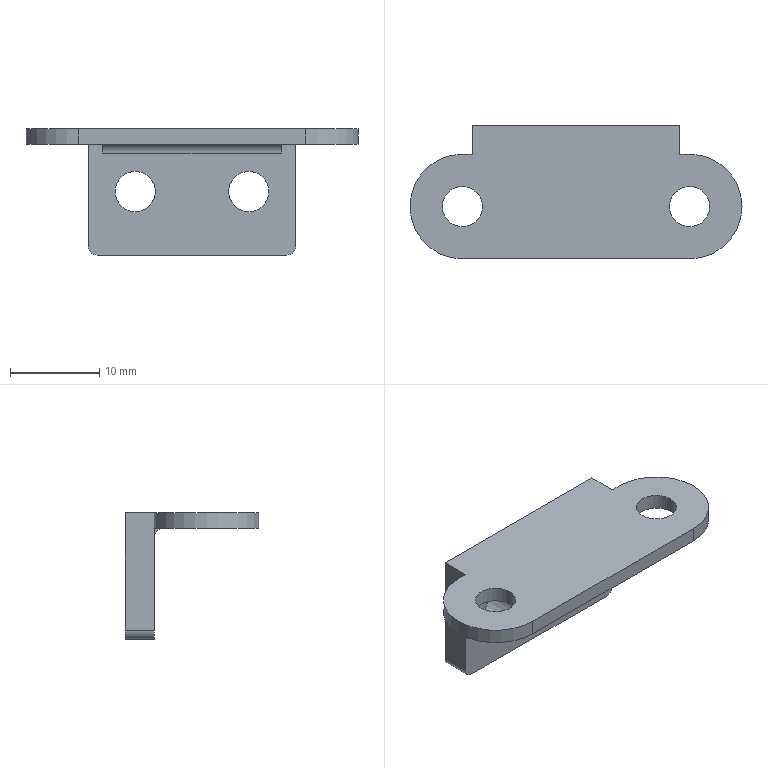Part | STEP file | CHAIN-04_1_02LT_1-2 | 1 solid | 26 faces | box 37.1 x 14.95 x 14.1 mm | volume 1597 mm3 | cylinder 14 | plane 12 | commonest cylinder face diameters 4.5 x8 2 x3 11.7 x3
STEP:
#1=CARTESIAN_POINT('',(-14.95,0.,0.));
#2=VERTEX_POINT('',#1);
#3=CARTESIAN_POINT('',(-10.45,0.,0.));
#4=VERTEX_POINT('',#3);
#5=CARTESIAN_POINT('',(-12.7,0.,0.));
#6=DIRECTION('',(0.,0.,1.));
#7=DIRECTION('',(1.,0.,0.));
#8=AXIS2_PLACEMENT_3D('',#5,#6,#7);
#9=CIRCLE('',#8,2.25);
#10=EDGE_CURVE('',#2,#4,#9,.T.);
#11=ORIENTED_EDGE('',*,*,#10,.F.);
#12=CARTESIAN_POINT('',(-14.95,0.,1.7));
#13=VERTEX_POINT('',#12);
#14=CARTESIAN_POINT('',(-14.95,0.,0.));
#15=DIRECTION('',(0.,0.,1.));
#16=VECTOR('',#15,1000.);
#17=LINE('',#14,#16);
#18=EDGE_CURVE('',#2,#13,#17,.T.);
#19=ORIENTED_EDGE('',*,*,#18,.T.);
#20=CARTESIAN_POINT('',(-10.45,0.,1.7));
#21=VERTEX_POINT('',#20);
#22=CARTESIAN_POINT('',(-12.7,0.,1.7));
#23=DIRECTION('',(0.,0.,-1.));
#24=DIRECTION('',(1.,0.,0.));
#25=AXIS2_PLACEMENT_3D('',#22,#23,#24);
#26=CIRCLE('',#25,2.25);
#27=EDGE_CURVE('',#21,#13,#26,.T.);
#28=ORIENTED_EDGE('',*,*,#27,.F.);
#29=CARTESIAN_POINT('',(-10.45,0.,0.));
#30=DIRECTION('',(0.,0.,1.));
#31=VECTOR('',#30,1000.);
#32=LINE('',#29,#31);
#33=EDGE_CURVE('',#4,#21,#32,.T.);
#34=ORIENTED_EDGE('',*,*,#33,.F.);
#35=EDGE_LOOP('',(#11,#19,#28,#34));
#36=FACE_OUTER_BOUND('',#35,.T.);
#37=CARTESIAN_POINT('',(-12.7,0.,0.));
#38=DIRECTION('',(0.,0.,1.));
#39=DIRECTION('',(1.,0.,0.));
#40=AXIS2_PLACEMENT_3D('',#37,#38,#39);
#41=CYLINDRICAL_SURFACE('',#40,2.25);
#42=ADVANCED_FACE('',(#36),#41,.F.);
#43=CARTESIAN_POINT('',(10.45,0.,0.));
#44=VERTEX_POINT('',#43);
#45=CARTESIAN_POINT('',(14.95,0.,0.));
#46=VERTEX_POINT('',#45);
#47=CARTESIAN_POINT('',(12.7,0.,0.));
#48=DIRECTION('',(0.,0.,1.));
#49=DIRECTION('',(1.,0.,0.));
#50=AXIS2_PLACEMENT_3D('',#47,#48,#49);
#51=CIRCLE('',#50,2.25);
#52=EDGE_CURVE('',#44,#46,#51,.T.);
#53=ORIENTED_EDGE('',*,*,#52,.F.);
#54=CARTESIAN_POINT('',(10.45,0.,1.7));
#55=VERTEX_POINT('',#54);
#56=CARTESIAN_POINT('',(10.45,0.,0.));
#57=DIRECTION('',(0.,0.,1.));
#58=VECTOR('',#57,1000.);
#59=LINE('',#56,#58);
#60=EDGE_CURVE('',#44,#55,#59,.T.);
#61=ORIENTED_EDGE('',*,*,#60,.T.);
#62=CARTESIAN_POINT('',(14.95,0.,1.7));
#63=VERTEX_POINT('',#62);
#64=CARTESIAN_POINT('',(12.7,0.,1.7));
#65=DIRECTION('',(0.,0.,-1.));
#66=DIRECTION('',(1.,0.,0.));
#67=AXIS2_PLACEMENT_3D('',#64,#65,#66);
#68=CIRCLE('',#67,2.25);
#69=EDGE_CURVE('',#63,#55,#68,.T.);
#70=ORIENTED_EDGE('',*,*,#69,.F.);
#71=CARTESIAN_POINT('',(14.95,0.,0.));
#72=DIRECTION('',(0.,0.,1.));
#73=VECTOR('',#72,1000.);
#74=LINE('',#71,#73);
#75=EDGE_CURVE('',#46,#63,#74,.T.);
#76=ORIENTED_EDGE('',*,*,#75,.F.);
#77=EDGE_LOOP('',(#53,#61,#70,#76));
#78=FACE_OUTER_BOUND('',#77,.T.);
#79=CARTESIAN_POINT('',(12.7,0.,0.));
#80=DIRECTION('',(0.,0.,1.));
#81=DIRECTION('',(1.,0.,0.));
#82=AXIS2_PLACEMENT_3D('',#79,#80,#81);
#83=CYLINDRICAL_SURFACE('',#82,2.25);
#84=ADVANCED_FACE('',(#78),#83,.F.);
#85=CARTESIAN_POINT('',(12.7,-5.85,0.));
#86=VERTEX_POINT('',#85);
#87=CARTESIAN_POINT('',(18.55,0.,0.));
#88=VERTEX_POINT('',#87);
#89=CARTESIAN_POINT('',(12.7,0.,0.));
#90=DIRECTION('',(0.,0.,1.));
#91=DIRECTION('',(1.,0.,0.));
#92=AXIS2_PLACEMENT_3D('',#89,#90,#91);
#93=CIRCLE('',#92,5.85);
#94=EDGE_CURVE('',#86,#88,#93,.T.);
#95=ORIENTED_EDGE('',*,*,#94,.T.);
#96=CARTESIAN_POINT('',(18.55,0.,1.7));
#97=VERTEX_POINT('',#96);
#98=CARTESIAN_POINT('',(18.55,0.,0.));
#99=DIRECTION('',(0.,0.,1.));
#100=VECTOR('',#99,1000.);
#101=LINE('',#98,#100);
#102=EDGE_CURVE('',#88,#97,#101,.T.);
#103=ORIENTED_EDGE('',*,*,#102,.T.);
#104=CARTESIAN_POINT('',(12.7,-5.85,1.7));
#105=VERTEX_POINT('',#104);
#106=CARTESIAN_POINT('',(12.7,0.,1.7));
#107=DIRECTION('',(0.,0.,1.));
#108=DIRECTION('',(1.,0.,0.));
#109=AXIS2_PLACEMENT_3D('',#106,#107,#108);
#110=CIRCLE('',#109,5.85);
#111=EDGE_CURVE('',#105,#97,#110,.T.);
#112=ORIENTED_EDGE('',*,*,#111,.F.);
#113=CARTESIAN_POINT('',(12.7,-5.85,0.));
#114=DIRECTION('',(0.,0.,-1.));
#115=VECTOR('',#114,1000.);
#116=LINE('',#113,#115);
#117=EDGE_CURVE('',#105,#86,#116,.T.);
#118=ORIENTED_EDGE('',*,*,#117,.T.);
#119=EDGE_LOOP('',(#95,#103,#112,#118));
#120=FACE_OUTER_BOUND('',#119,.T.);
#121=CARTESIAN_POINT('',(12.7,0.,0.));
#122=DIRECTION('',(0.,0.,1.));
#123=DIRECTION('',(1.,0.,0.));
#124=AXIS2_PLACEMENT_3D('',#121,#122,#123);
#125=CYLINDRICAL_SURFACE('',#124,5.85);
#126=ADVANCED_FACE('',(#120),#125,.T.);
#127=CARTESIAN_POINT('',(6.35,5.85,-3.05));
#128=VERTEX_POINT('',#127);
#129=CARTESIAN_POINT('',(6.35,5.85,-7.55));
#130=VERTEX_POINT('',#129);
#131=CARTESIAN_POINT('',(6.35,5.85,-5.3));
#132=DIRECTION('',(0.,-1.,0.));
#133=DIRECTION('',(0.,0.,1.));
#134=AXIS2_PLACEMENT_3D('',#131,#132,#133);
#135=CIRCLE('',#134,2.25);
#136=EDGE_CURVE('',#128,#130,#135,.T.);
#137=ORIENTED_EDGE('',*,*,#136,.T.);
#138=CARTESIAN_POINT('',(6.35,9.1,-7.55));
#139=VERTEX_POINT('',#138);
#140=CARTESIAN_POINT('',(6.35,9.1,-7.55));
#141=DIRECTION('',(0.,1.,0.));
#142=VECTOR('',#141,1000.);
#143=LINE('',#140,#142);
#144=EDGE_CURVE('',#130,#139,#143,.T.);
#145=ORIENTED_EDGE('',*,*,#144,.T.);
#146=CARTESIAN_POINT('',(6.35,9.1,-3.05));
#147=VERTEX_POINT('',#146);
#148=CARTESIAN_POINT('',(6.35,9.1,-5.3));
#149=DIRECTION('',(0.,1.,0.));
#150=DIRECTION('',(0.,0.,1.));
#151=AXIS2_PLACEMENT_3D('',#148,#149,#150);
#152=CIRCLE('',#151,2.25);
#153=EDGE_CURVE('',#139,#147,#152,.T.);
#154=ORIENTED_EDGE('',*,*,#153,.T.);
#155=CARTESIAN_POINT('',(6.35,9.1,-3.05));
#156=DIRECTION('',(0.,1.,0.));
#157=VECTOR('',#156,1000.);
#158=LINE('',#155,#157);
#159=EDGE_CURVE('',#128,#147,#158,.T.);
#160=ORIENTED_EDGE('',*,*,#159,.F.);
#161=EDGE_LOOP('',(#137,#145,#154,#160));
#162=FACE_OUTER_BOUND('',#161,.T.);
#163=CARTESIAN_POINT('',(6.35,9.1,-5.3));
#164=DIRECTION('',(0.,1.,0.));
#165=DIRECTION('',(0.,0.,1.));
#166=AXIS2_PLACEMENT_3D('',#163,#164,#165);
#167=CYLINDRICAL_SURFACE('',#166,2.25);
#168=ADVANCED_FACE('',(#162),#167,.F.);
#169=CARTESIAN_POINT('',(-6.35,5.85,-3.05));
#170=VERTEX_POINT('',#169);
#171=CARTESIAN_POINT('',(-6.35,5.85,-7.55));
#172=VERTEX_POINT('',#171);
#173=CARTESIAN_POINT('',(-6.35,5.85,-5.3));
#174=DIRECTION('',(0.,-1.,0.));
#175=DIRECTION('',(0.,0.,1.));
#176=AXIS2_PLACEMENT_3D('',#173,#174,#175);
#177=CIRCLE('',#176,2.25);
#178=EDGE_CURVE('',#170,#172,#177,.T.);
#179=ORIENTED_EDGE('',*,*,#178,.T.);
#180=CARTESIAN_POINT('',(-6.35,9.1,-7.55));
#181=VERTEX_POINT('',#180);
#182=CARTESIAN_POINT('',(-6.35,9.1,-7.55));
#183=DIRECTION('',(0.,1.,0.));
#184=VECTOR('',#183,1000.);
#185=LINE('',#182,#184);
#186=EDGE_CURVE('',#172,#181,#185,.T.);
#187=ORIENTED_EDGE('',*,*,#186,.T.);
#188=CARTESIAN_POINT('',(-6.35,9.1,-3.05));
#189=VERTEX_POINT('',#188);
#190=CARTESIAN_POINT('',(-6.35,9.1,-5.3));
#191=DIRECTION('',(0.,1.,0.));
#192=DIRECTION('',(0.,0.,1.));
#193=AXIS2_PLACEMENT_3D('',#190,#191,#192);
#194=CIRCLE('',#193,2.25);
#195=EDGE_CURVE('',#181,#189,#194,.T.);
#196=ORIENTED_EDGE('',*,*,#195,.T.);
#197=CARTESIAN_POINT('',(-6.35,9.1,-3.05));
#198=DIRECTION('',(0.,1.,0.));
#199=VECTOR('',#198,1000.);
#200=LINE('',#197,#199);
#201=EDGE_CURVE('',#170,#189,#200,.T.);
#202=ORIENTED_EDGE('',*,*,#201,.F.);
#203=EDGE_LOOP('',(#179,#187,#196,#202));
#204=FACE_OUTER_BOUND('',#203,.T.);
#205=CARTESIAN_POINT('',(-6.35,9.1,-5.3));
#206=DIRECTION('',(0.,1.,0.));
#207=DIRECTION('',(0.,0.,1.));
#208=AXIS2_PLACEMENT_3D('',#205,#206,#207);
#209=CYLINDRICAL_SURFACE('',#208,2.25);
#210=ADVANCED_FACE('',(#204),#209,.F.);
#211=ORIENTED_EDGE('',*,*,#27,.T.);
#212=CARTESIAN_POINT('',(-12.7,0.,1.7));
#213=DIRECTION('',(0.,0.,-1.));
#214=DIRECTION('',(1.,0.,0.));
#215=AXIS2_PLACEMENT_3D('',#212,#213,#214);
#216=CIRCLE('',#215,2.25);
#217=EDGE_CURVE('',#13,#21,#216,.T.);
#218=ORIENTED_EDGE('',*,*,#217,.T.);
#219=EDGE_LOOP('',(#211,#218));
#220=FACE_BOUND('',#219,.T.);
#221=ORIENTED_EDGE('',*,*,#69,.T.);
#222=CARTESIAN_POINT('',(12.7,0.,1.7));
#223=DIRECTION('',(0.,0.,-1.));
#224=DIRECTION('',(1.,0.,0.));
#225=AXIS2_PLACEMENT_3D('',#222,#223,#224);
#226=CIRCLE('',#225,2.25);
#227=EDGE_CURVE('',#55,#63,#226,.T.);
#228=ORIENTED_EDGE('',*,*,#227,.T.);
#229=EDGE_LOOP('',(#221,#228));
#230=FACE_BOUND('',#229,.T.);
#231=CARTESIAN_POINT('',(11.6,9.1,1.7));
#232=VERTEX_POINT('',#231);
#233=CARTESIAN_POINT('',(-11.6,9.1,1.7));
#234=VERTEX_POINT('',#233);
#235=CARTESIAN_POINT('',(0.,9.1,1.7));
#236=DIRECTION('',(-1.,0.,0.));
#237=VECTOR('',#236,1000.);
#238=LINE('',#235,#237);
#239=EDGE_CURVE('',#232,#234,#238,.T.);
#240=ORIENTED_EDGE('',*,*,#239,.T.);
#241=CARTESIAN_POINT('',(-11.6,5.85,1.7));
#242=VERTEX_POINT('',#241);
#243=CARTESIAN_POINT('',(-11.6,0.,1.7));
#244=DIRECTION('',(0.,-1.,0.));
#245=VECTOR('',#244,1000.);
#246=LINE('',#243,#245);
#247=EDGE_CURVE('',#234,#242,#246,.T.);
#248=ORIENTED_EDGE('',*,*,#247,.T.);
#249=CARTESIAN_POINT('',(-12.7,5.85,1.7));
#250=VERTEX_POINT('',#249);
#251=CARTESIAN_POINT('',(0.,5.85,1.7));
#252=DIRECTION('',(-1.,0.,0.));
#253=VECTOR('',#252,1000.);
#254=LINE('',#251,#253);
#255=EDGE_CURVE('',#242,#250,#254,.T.);
#256=ORIENTED_EDGE('',*,*,#255,.T.);
#257=CARTESIAN_POINT('',(-12.7,-5.85,1.7));
#258=VERTEX_POINT('',#257);
#259=CARTESIAN_POINT('',(-12.7,0.,1.7));
#260=DIRECTION('',(0.,0.,1.));
#261=DIRECTION('',(1.,0.,0.));
#262=AXIS2_PLACEMENT_3D('',#259,#260,#261);
#263=CIRCLE('',#262,5.85);
#264=EDGE_CURVE('',#250,#258,#263,.T.);
#265=ORIENTED_EDGE('',*,*,#264,.T.);
#266=CARTESIAN_POINT('',(0.,-5.85,1.7));
#267=DIRECTION('',(1.,0.,0.));
#268=VECTOR('',#267,1000.);
#269=LINE('',#266,#268);
#270=EDGE_CURVE('',#258,#105,#269,.T.);
#271=ORIENTED_EDGE('',*,*,#270,.T.);
#272=ORIENTED_EDGE('',*,*,#111,.T.);
#273=CARTESIAN_POINT('',(12.7,5.85,1.7));
#274=VERTEX_POINT('',#273);
#275=CARTESIAN_POINT('',(12.7,0.,1.7));
#276=DIRECTION('',(0.,0.,1.));
#277=DIRECTION('',(1.,0.,0.));
#278=AXIS2_PLACEMENT_3D('',#275,#276,#277);
#279=CIRCLE('',#278,5.85);
#280=EDGE_CURVE('',#97,#274,#279,.T.);
#281=ORIENTED_EDGE('',*,*,#280,.T.);
#282=CARTESIAN_POINT('',(11.6,5.85,1.7));
#283=VERTEX_POINT('',#282);
#284=CARTESIAN_POINT('',(0.,5.85,1.7));
#285=DIRECTION('',(-1.,0.,0.));
#286=VECTOR('',#285,1000.);
#287=LINE('',#284,#286);
#288=EDGE_CURVE('',#274,#283,#287,.T.);
#289=ORIENTED_EDGE('',*,*,#288,.T.);
#290=CARTESIAN_POINT('',(11.6,0.,1.7));
#291=DIRECTION('',(0.,1.,0.));
#292=VECTOR('',#291,1000.);
#293=LINE('',#290,#292);
#294=EDGE_CURVE('',#283,#232,#293,.T.);
#295=ORIENTED_EDGE('',*,*,#294,.T.);
#296=EDGE_LOOP('',(#240,#248,#256,#265,#271,#272,#281,#289,#295));
#297=FACE_OUTER_BOUND('',#296,.T.);
#298=CARTESIAN_POINT('',(0.,0.,1.7));
#299=DIRECTION('',(0.,0.,1.));
#300=DIRECTION('',(1.,0.,0.));
#301=AXIS2_PLACEMENT_3D('',#298,#299,#300);
#302=PLANE('',#301);
#303=ADVANCED_FACE('',(#220,#230,#297),#302,.T.);
#304=ORIENTED_EDGE('',*,*,#18,.F.);
#305=CARTESIAN_POINT('',(-12.7,0.,0.));
#306=DIRECTION('',(0.,0.,1.));
#307=DIRECTION('',(1.,0.,0.));
#308=AXIS2_PLACEMENT_3D('',#305,#306,#307);
#309=CIRCLE('',#308,2.25);
#310=EDGE_CURVE('',#4,#2,#309,.T.);
#311=ORIENTED_EDGE('',*,*,#310,.F.);
#312=ORIENTED_EDGE('',*,*,#33,.T.);
#313=ORIENTED_EDGE('',*,*,#217,.F.);
#314=EDGE_LOOP('',(#304,#311,#312,#313));
#315=FACE_OUTER_BOUND('',#314,.T.);
#316=CARTESIAN_POINT('',(-12.7,0.,0.));
#317=DIRECTION('',(0.,0.,1.));
#318=DIRECTION('',(1.,0.,0.));
#319=AXIS2_PLACEMENT_3D('',#316,#317,#318);
#320=CYLINDRICAL_SURFACE('',#319,2.25);
#321=ADVANCED_FACE('',(#315),#320,.F.);
#322=ORIENTED_EDGE('',*,*,#60,.F.);
#323=CARTESIAN_POINT('',(12.7,0.,0.));
#324=DIRECTION('',(0.,0.,1.));
#325=DIRECTION('',(1.,0.,0.));
#326=AXIS2_PLACEMENT_3D('',#323,#324,#325);
#327=CIRCLE('',#326,2.25);
#328=EDGE_CURVE('',#46,#44,#327,.T.);
#329=ORIENTED_EDGE('',*,*,#328,.F.);
#330=ORIENTED_EDGE('',*,*,#75,.T.);
#331=ORIENTED_EDGE('',*,*,#227,.F.);
#332=EDGE_LOOP('',(#322,#329,#330,#331));
#333=FACE_OUTER_BOUND('',#332,.T.);
#334=CARTESIAN_POINT('',(12.7,0.,0.));
#335=DIRECTION('',(0.,0.,1.));
#336=DIRECTION('',(1.,0.,0.));
#337=AXIS2_PLACEMENT_3D('',#334,#335,#336);
#338=CYLINDRICAL_SURFACE('',#337,2.25);
#339=ADVANCED_FACE('',(#333),#338,.F.);
#340=CARTESIAN_POINT('',(-11.6,5.85,0.));
#341=VERTEX_POINT('',#340);
#342=CARTESIAN_POINT('',(-11.6,5.85,-11.4));
#343=VERTEX_POINT('',#342);
#344=CARTESIAN_POINT('',(-11.6,5.85,1.7));
#345=DIRECTION('',(0.,0.,-1.));
#346=VECTOR('',#345,1000.);
#347=LINE('',#344,#346);
#348=EDGE_CURVE('',#341,#343,#347,.T.);
#349=ORIENTED_EDGE('',*,*,#348,.F.);
#350=CARTESIAN_POINT('',(-11.6,5.85,1.7));
#351=DIRECTION('',(0.,0.,-1.));
#352=VECTOR('',#351,1000.);
#353=LINE('',#350,#352);
#354=EDGE_CURVE('',#242,#341,#353,.T.);
#355=ORIENTED_EDGE('',*,*,#354,.F.);
#356=ORIENTED_EDGE('',*,*,#247,.F.);
#357=CARTESIAN_POINT('',(-11.6,9.1,-11.4));
#358=VERTEX_POINT('',#357);
#359=CARTESIAN_POINT('',(-11.6,9.1,1.7));
#360=DIRECTION('',(0.,0.,1.));
#361=VECTOR('',#360,1000.);
#362=LINE('',#359,#361);
#363=EDGE_CURVE('',#358,#234,#362,.T.);
#364=ORIENTED_EDGE('',*,*,#363,.F.);
#365=CARTESIAN_POINT('',(-11.6,9.1,-11.4));
#366=DIRECTION('',(0.,1.,0.));
#367=VECTOR('',#366,1000.);
#368=LINE('',#365,#367);
#369=EDGE_CURVE('',#343,#358,#368,.T.);
#370=ORIENTED_EDGE('',*,*,#369,.F.);
#371=EDGE_LOOP('',(#349,#355,#356,#364,#370));
#372=FACE_OUTER_BOUND('',#371,.T.);
#373=CARTESIAN_POINT('',(-11.6,9.1,1.7));
#374=DIRECTION('',(1.,0.,0.));
#375=DIRECTION('',(0.,0.,-1.));
#376=AXIS2_PLACEMENT_3D('',#373,#374,#375);
#377=PLANE('',#376);
#378=ADVANCED_FACE('',(#372),#377,.F.);
#379=CARTESIAN_POINT('',(6.35,9.1,-5.3));
#380=DIRECTION('',(0.,1.,0.));
#381=DIRECTION('',(0.,0.,1.));
#382=AXIS2_PLACEMENT_3D('',#379,#380,#381);
#383=CIRCLE('',#382,2.25);
#384=EDGE_CURVE('',#147,#139,#383,.T.);
#385=ORIENTED_EDGE('',*,*,#384,.F.);
#386=ORIENTED_EDGE('',*,*,#153,.F.);
#387=EDGE_LOOP('',(#385,#386));
#388=FACE_BOUND('',#387,.T.);
#389=CARTESIAN_POINT('',(-6.35,9.1,-5.3));
#390=DIRECTION('',(0.,1.,0.));
#391=DIRECTION('',(0.,0.,1.));
#392=AXIS2_PLACEMENT_3D('',#389,#390,#391);
#393=CIRCLE('',#392,2.25);
#394=EDGE_CURVE('',#189,#181,#393,.T.);
#395=ORIENTED_EDGE('',*,*,#394,.F.);
#396=ORIENTED_EDGE('',*,*,#195,.F.);
#397=EDGE_LOOP('',(#395,#396));
#398=FACE_BOUND('',#397,.T.);
#399=CARTESIAN_POINT('',(-10.6,9.1,-12.4));
#400=VERTEX_POINT('',#399);
#401=CARTESIAN_POINT('',(10.6,9.1,-12.4));
#402=VERTEX_POINT('',#401);
#403=CARTESIAN_POINT('',(-11.6,9.1,-12.4));
#404=DIRECTION('',(1.,0.,0.));
#405=VECTOR('',#404,1000.);
#406=LINE('',#403,#405);
#407=EDGE_CURVE('',#400,#402,#406,.T.);
#408=ORIENTED_EDGE('',*,*,#407,.F.);
#409=CARTESIAN_POINT('',(-10.6,9.1,-11.4));
#410=DIRECTION('',(0.,-1.,0.));
#411=DIRECTION('',(0.,0.,-1.));
#412=AXIS2_PLACEMENT_3D('',#409,#410,#411);
#413=CIRCLE('',#412,1.);
#414=EDGE_CURVE('',#358,#400,#413,.T.);
#415=ORIENTED_EDGE('',*,*,#414,.F.);
#416=ORIENTED_EDGE('',*,*,#363,.T.);
#417=ORIENTED_EDGE('',*,*,#239,.F.);
#418=CARTESIAN_POINT('',(11.6,9.1,-11.4));
#419=VERTEX_POINT('',#418);
#420=CARTESIAN_POINT('',(11.6,9.1,-12.4));
#421=DIRECTION('',(0.,0.,1.));
#422=VECTOR('',#421,1000.);
#423=LINE('',#420,#422);
#424=EDGE_CURVE('',#419,#232,#423,.T.);
#425=ORIENTED_EDGE('',*,*,#424,.F.);
#426=CARTESIAN_POINT('',(10.6,9.1,-11.4));
#427=DIRECTION('',(0.,-1.,0.));
#428=DIRECTION('',(0.,0.,-1.));
#429=AXIS2_PLACEMENT_3D('',#426,#427,#428);
#430=CIRCLE('',#429,1.);
#431=EDGE_CURVE('',#402,#419,#430,.T.);
#432=ORIENTED_EDGE('',*,*,#431,.F.);
#433=EDGE_LOOP('',(#408,#415,#416,#417,#425,#432));
#434=FACE_OUTER_BOUND('',#433,.T.);
#435=CARTESIAN_POINT('',(-11.6,9.1,-12.4));
#436=DIRECTION('',(0.,-1.,0.));
#437=DIRECTION('',(0.,0.,-1.));
#438=AXIS2_PLACEMENT_3D('',#435,#436,#437);
#439=PLANE('',#438);
#440=ADVANCED_FACE('',(#388,#398,#434),#439,.F.);
#441=ORIENTED_EDGE('',*,*,#424,.T.);
#442=ORIENTED_EDGE('',*,*,#294,.F.);
#443=CARTESIAN_POINT('',(11.6,5.85,0.));
#444=VERTEX_POINT('',#443);
#445=CARTESIAN_POINT('',(11.6,5.85,1.7));
#446=DIRECTION('',(0.,0.,1.));
#447=VECTOR('',#446,1000.);
#448=LINE('',#445,#447);
#449=EDGE_CURVE('',#444,#283,#448,.T.);
#450=ORIENTED_EDGE('',*,*,#449,.F.);
#451=CARTESIAN_POINT('',(11.6,5.85,-11.4));
#452=VERTEX_POINT('',#451);
#453=CARTESIAN_POINT('',(11.6,5.85,1.7));
#454=DIRECTION('',(0.,0.,1.));
#455=VECTOR('',#454,1000.);
#456=LINE('',#453,#455);
#457=EDGE_CURVE('',#452,#444,#456,.T.);
#458=ORIENTED_EDGE('',*,*,#457,.F.);
#459=CARTESIAN_POINT('',(11.6,9.1,-11.4));
#460=DIRECTION('',(0.,-1.,0.));
#461=VECTOR('',#460,1000.);
#462=LINE('',#459,#461);
#463=EDGE_CURVE('',#419,#452,#462,.T.);
#464=ORIENTED_EDGE('',*,*,#463,.F.);
#465=EDGE_LOOP('',(#441,#442,#450,#458,#464));
#466=FACE_OUTER_BOUND('',#465,.T.);
#467=CARTESIAN_POINT('',(11.6,9.1,1.7));
#468=DIRECTION('',(-1.,0.,0.));
#469=DIRECTION('',(0.,0.,1.));
#470=AXIS2_PLACEMENT_3D('',#467,#468,#469);
#471=PLANE('',#470);
#472=ADVANCED_FACE('',(#466),#471,.F.);
#473=CARTESIAN_POINT('',(12.7,5.85,0.));
#474=VERTEX_POINT('',#473);
#475=CARTESIAN_POINT('',(12.7,5.85,0.));
#476=DIRECTION('',(0.,0.,-1.));
#477=VECTOR('',#476,1000.);
#478=LINE('',#475,#477);
#479=EDGE_CURVE('',#274,#474,#478,.T.);
#480=ORIENTED_EDGE('',*,*,#479,.T.);
#481=CARTESIAN_POINT('',(12.7,5.85,0.));
#482=DIRECTION('',(-1.,0.,0.));
#483=VECTOR('',#482,1000.);
#484=LINE('',#481,#483);
#485=EDGE_CURVE('',#474,#444,#484,.T.);
#486=ORIENTED_EDGE('',*,*,#485,.T.);
#487=ORIENTED_EDGE('',*,*,#449,.T.);
#488=ORIENTED_EDGE('',*,*,#288,.F.);
#489=EDGE_LOOP('',(#480,#486,#487,#488));
#490=FACE_OUTER_BOUND('',#489,.T.);
#491=CARTESIAN_POINT('',(12.7,5.85,0.));
#492=DIRECTION('',(0.,1.,0.));
#493=DIRECTION('',(0.,0.,1.));
#494=AXIS2_PLACEMENT_3D('',#491,#492,#493);
#495=PLANE('',#494);
#496=ADVANCED_FACE('',(#490),#495,.T.);
#497=ORIENTED_EDGE('',*,*,#102,.F.);
#498=CARTESIAN_POINT('',(12.7,0.,0.));
#499=DIRECTION('',(0.,0.,1.));
#500=DIRECTION('',(1.,0.,0.));
#501=AXIS2_PLACEMENT_3D('',#498,#499,#500);
#502=CIRCLE('',#501,5.85);
#503=EDGE_CURVE('',#88,#474,#502,.T.);
#504=ORIENTED_EDGE('',*,*,#503,.T.);
#505=ORIENTED_EDGE('',*,*,#479,.F.);
#506=ORIENTED_EDGE('',*,*,#280,.F.);
#507=EDGE_LOOP('',(#497,#504,#505,#506));
#508=FACE_OUTER_BOUND('',#507,.T.);
#509=CARTESIAN_POINT('',(12.7,0.,0.));
#510=DIRECTION('',(0.,0.,1.));
#511=DIRECTION('',(1.,0.,0.));
#512=AXIS2_PLACEMENT_3D('',#509,#510,#511);
#513=CYLINDRICAL_SURFACE('',#512,5.85);
#514=ADVANCED_FACE('',(#508),#513,.T.);
#515=ORIENTED_EDGE('',*,*,#117,.F.);
#516=ORIENTED_EDGE('',*,*,#270,.F.);
#517=CARTESIAN_POINT('',(-12.7,-5.85,0.));
#518=VERTEX_POINT('',#517);
#519=CARTESIAN_POINT('',(-12.7,-5.85,0.));
#520=DIRECTION('',(0.,0.,-1.));
#521=VECTOR('',#520,1000.);
#522=LINE('',#519,#521);
#523=EDGE_CURVE('',#258,#518,#522,.T.);
#524=ORIENTED_EDGE('',*,*,#523,.T.);
#525=CARTESIAN_POINT('',(-12.7,-5.85,0.));
#526=DIRECTION('',(1.,0.,0.));
#527=VECTOR('',#526,1000.);
#528=LINE('',#525,#527);
#529=EDGE_CURVE('',#518,#86,#528,.T.);
#530=ORIENTED_EDGE('',*,*,#529,.T.);
#531=EDGE_LOOP('',(#515,#516,#524,#530));
#532=FACE_OUTER_BOUND('',#531,.T.);
#533=CARTESIAN_POINT('',(-12.7,-5.85,0.));
#534=DIRECTION('',(0.,-1.,0.));
#535=DIRECTION('',(0.,0.,-1.));
#536=AXIS2_PLACEMENT_3D('',#533,#534,#535);
#537=PLANE('',#536);
#538=ADVANCED_FACE('',(#532),#537,.T.);
#539=ORIENTED_EDGE('',*,*,#523,.F.);
#540=ORIENTED_EDGE('',*,*,#264,.F.);
#541=CARTESIAN_POINT('',(-12.7,5.85,0.));
#542=VERTEX_POINT('',#541);
#543=CARTESIAN_POINT('',(-12.7,5.85,0.));
#544=DIRECTION('',(0.,0.,-1.));
#545=VECTOR('',#544,1000.);
#546=LINE('',#543,#545);
#547=EDGE_CURVE('',#250,#542,#546,.T.);
#548=ORIENTED_EDGE('',*,*,#547,.T.);
#549=CARTESIAN_POINT('',(-12.7,0.,0.));
#550=DIRECTION('',(0.,0.,1.));
#551=DIRECTION('',(1.,0.,0.));
#552=AXIS2_PLACEMENT_3D('',#549,#550,#551);
#553=CIRCLE('',#552,5.85);
#554=EDGE_CURVE('',#542,#518,#553,.T.);
#555=ORIENTED_EDGE('',*,*,#554,.T.);
#556=EDGE_LOOP('',(#539,#540,#548,#555));
#557=FACE_OUTER_BOUND('',#556,.T.);
#558=CARTESIAN_POINT('',(-12.7,0.,0.));
#559=DIRECTION('',(0.,0.,1.));
#560=DIRECTION('',(1.,0.,0.));
#561=AXIS2_PLACEMENT_3D('',#558,#559,#560);
#562=CYLINDRICAL_SURFACE('',#561,5.85);
#563=ADVANCED_FACE('',(#557),#562,.T.);
#564=ORIENTED_EDGE('',*,*,#547,.F.);
#565=ORIENTED_EDGE('',*,*,#255,.F.);
#566=ORIENTED_EDGE('',*,*,#354,.T.);
#567=CARTESIAN_POINT('',(12.7,5.85,0.));
#568=DIRECTION('',(-1.,0.,0.));
#569=VECTOR('',#568,1000.);
#570=LINE('',#567,#569);
#571=EDGE_CURVE('',#341,#542,#570,.T.);
#572=ORIENTED_EDGE('',*,*,#571,.T.);
#573=EDGE_LOOP('',(#564,#565,#566,#572));
#574=FACE_OUTER_BOUND('',#573,.T.);
#575=CARTESIAN_POINT('',(12.7,5.85,0.));
#576=DIRECTION('',(0.,1.,0.));
#577=DIRECTION('',(0.,0.,1.));
#578=AXIS2_PLACEMENT_3D('',#575,#576,#577);
#579=PLANE('',#578);
#580=ADVANCED_FACE('',(#574),#579,.T.);
#581=ORIENTED_EDGE('',*,*,#310,.T.);
#582=ORIENTED_EDGE('',*,*,#10,.T.);
#583=EDGE_LOOP('',(#581,#582));
#584=FACE_BOUND('',#583,.T.);
#585=ORIENTED_EDGE('',*,*,#328,.T.);
#586=ORIENTED_EDGE('',*,*,#52,.T.);
#587=EDGE_LOOP('',(#585,#586));
#588=FACE_BOUND('',#587,.T.);
#589=ORIENTED_EDGE('',*,*,#554,.F.);
#590=ORIENTED_EDGE('',*,*,#571,.F.);
#591=CARTESIAN_POINT('',(-10.,5.85,0.));
#592=VERTEX_POINT('',#591);
#593=CARTESIAN_POINT('',(0.,5.85,0.));
#594=DIRECTION('',(-1.,0.,0.));
#595=VECTOR('',#594,1000.);
#596=LINE('',#593,#595);
#597=EDGE_CURVE('',#592,#341,#596,.T.);
#598=ORIENTED_EDGE('',*,*,#597,.F.);
#599=CARTESIAN_POINT('',(-10.,4.85,0.));
#600=VERTEX_POINT('',#599);
#601=CARTESIAN_POINT('',(-10.,0.,0.));
#602=DIRECTION('',(0.,1.,0.));
#603=VECTOR('',#602,1000.);
#604=LINE('',#601,#603);
#605=EDGE_CURVE('',#600,#592,#604,.T.);
#606=ORIENTED_EDGE('',*,*,#605,.F.);
#607=CARTESIAN_POINT('',(10.,4.85,0.));
#608=VERTEX_POINT('',#607);
#609=CARTESIAN_POINT('',(0.,4.85,0.));
#610=DIRECTION('',(-1.,0.,0.));
#611=VECTOR('',#610,1000.);
#612=LINE('',#609,#611);
#613=EDGE_CURVE('',#608,#600,#612,.T.);
#614=ORIENTED_EDGE('',*,*,#613,.F.);
#615=CARTESIAN_POINT('',(10.,5.85,0.));
#616=VERTEX_POINT('',#615);
#617=CARTESIAN_POINT('',(10.,0.,0.));
#618=DIRECTION('',(0.,-1.,0.));
#619=VECTOR('',#618,1000.);
#620=LINE('',#617,#619);
#621=EDGE_CURVE('',#616,#608,#620,.T.);
#622=ORIENTED_EDGE('',*,*,#621,.F.);
#623=CARTESIAN_POINT('',(0.,5.85,0.));
#624=DIRECTION('',(-1.,0.,0.));
#625=VECTOR('',#624,1000.);
#626=LINE('',#623,#625);
#627=EDGE_CURVE('',#444,#616,#626,.T.);
#628=ORIENTED_EDGE('',*,*,#627,.F.);
#629=ORIENTED_EDGE('',*,*,#485,.F.);
#630=ORIENTED_EDGE('',*,*,#503,.F.);
#631=ORIENTED_EDGE('',*,*,#94,.F.);
#632=ORIENTED_EDGE('',*,*,#529,.F.);
#633=EDGE_LOOP('',(#589,#590,#598,#606,#614,#622,#628,#629,#630,#631,#632));
#634=FACE_OUTER_BOUND('',#633,.T.);
#635=CARTESIAN_POINT('',(0.,0.,0.));
#636=DIRECTION('',(0.,0.,1.));
#637=DIRECTION('',(1.,0.,0.));
#638=AXIS2_PLACEMENT_3D('',#635,#636,#637);
#639=PLANE('',#638);
#640=ADVANCED_FACE('',(#584,#588,#634),#639,.F.);
#641=ORIENTED_EDGE('',*,*,#369,.T.);
#642=ORIENTED_EDGE('',*,*,#414,.T.);
#643=CARTESIAN_POINT('',(-10.6,5.85,-12.4));
#644=VERTEX_POINT('',#643);
#645=CARTESIAN_POINT('',(-10.6,9.1,-12.4));
#646=DIRECTION('',(0.,-1.,0.));
#647=VECTOR('',#646,1000.);
#648=LINE('',#645,#647);
#649=EDGE_CURVE('',#400,#644,#648,.T.);
#650=ORIENTED_EDGE('',*,*,#649,.T.);
#651=CARTESIAN_POINT('',(-10.6,5.85,-11.4));
#652=DIRECTION('',(0.,1.,0.));
#653=DIRECTION('',(0.,0.,-1.));
#654=AXIS2_PLACEMENT_3D('',#651,#652,#653);
#655=CIRCLE('',#654,1.);
#656=EDGE_CURVE('',#644,#343,#655,.T.);
#657=ORIENTED_EDGE('',*,*,#656,.T.);
#658=EDGE_LOOP('',(#641,#642,#650,#657));
#659=FACE_OUTER_BOUND('',#658,.T.);
#660=CARTESIAN_POINT('',(-10.6,9.1,-11.4));
#661=DIRECTION('',(0.,-1.,0.));
#662=DIRECTION('',(0.,0.,-1.));
#663=AXIS2_PLACEMENT_3D('',#660,#661,#662);
#664=CYLINDRICAL_SURFACE('',#663,1.);
#665=ADVANCED_FACE('',(#659),#664,.T.);
#666=ORIENTED_EDGE('',*,*,#136,.F.);
#667=CARTESIAN_POINT('',(6.35,5.85,-5.3));
#668=DIRECTION('',(0.,-1.,0.));
#669=DIRECTION('',(0.,0.,1.));
#670=AXIS2_PLACEMENT_3D('',#667,#668,#669);
#671=CIRCLE('',#670,2.25);
#672=EDGE_CURVE('',#130,#128,#671,.T.);
#673=ORIENTED_EDGE('',*,*,#672,.F.);
#674=EDGE_LOOP('',(#666,#673));
#675=FACE_BOUND('',#674,.T.);
#676=ORIENTED_EDGE('',*,*,#178,.F.);
#677=CARTESIAN_POINT('',(-6.35,5.85,-5.3));
#678=DIRECTION('',(0.,-1.,0.));
#679=DIRECTION('',(0.,0.,1.));
#680=AXIS2_PLACEMENT_3D('',#677,#678,#679);
#681=CIRCLE('',#680,2.25);
#682=EDGE_CURVE('',#172,#170,#681,.T.);
#683=ORIENTED_EDGE('',*,*,#682,.F.);
#684=EDGE_LOOP('',(#676,#683));
#685=FACE_BOUND('',#684,.T.);
#686=ORIENTED_EDGE('',*,*,#457,.T.);
#687=ORIENTED_EDGE('',*,*,#627,.T.);
#688=CARTESIAN_POINT('',(10.,5.85,-1.));
#689=VERTEX_POINT('',#688);
#690=CARTESIAN_POINT('',(10.,5.85,0.));
#691=DIRECTION('',(0.,0.,1.));
#692=VECTOR('',#691,1000.);
#693=LINE('',#690,#692);
#694=EDGE_CURVE('',#689,#616,#693,.T.);
#695=ORIENTED_EDGE('',*,*,#694,.F.);
#696=CARTESIAN_POINT('',(-10.,5.85,-1.));
#697=VERTEX_POINT('',#696);
#698=CARTESIAN_POINT('',(0.,5.85,-1.));
#699=DIRECTION('',(1.,0.,0.));
#700=VECTOR('',#699,1000.);
#701=LINE('',#698,#700);
#702=EDGE_CURVE('',#697,#689,#701,.T.);
#703=ORIENTED_EDGE('',*,*,#702,.F.);
#704=CARTESIAN_POINT('',(-10.,5.85,0.));
#705=DIRECTION('',(0.,0.,-1.));
#706=VECTOR('',#705,1000.);
#707=LINE('',#704,#706);
#708=EDGE_CURVE('',#592,#697,#707,.T.);
#709=ORIENTED_EDGE('',*,*,#708,.F.);
#710=ORIENTED_EDGE('',*,*,#597,.T.);
#711=ORIENTED_EDGE('',*,*,#348,.T.);
#712=ORIENTED_EDGE('',*,*,#656,.F.);
#713=CARTESIAN_POINT('',(10.6,5.85,-12.4));
#714=VERTEX_POINT('',#713);
#715=CARTESIAN_POINT('',(0.,5.85,-12.4));
#716=DIRECTION('',(-1.,0.,0.));
#717=VECTOR('',#716,1000.);
#718=LINE('',#715,#717);
#719=EDGE_CURVE('',#714,#644,#718,.T.);
#720=ORIENTED_EDGE('',*,*,#719,.F.);
#721=CARTESIAN_POINT('',(10.6,5.85,-11.4));
#722=DIRECTION('',(0.,1.,0.));
#723=DIRECTION('',(0.,0.,-1.));
#724=AXIS2_PLACEMENT_3D('',#721,#722,#723);
#725=CIRCLE('',#724,1.);
#726=EDGE_CURVE('',#452,#714,#725,.T.);
#727=ORIENTED_EDGE('',*,*,#726,.F.);
#728=EDGE_LOOP('',(#686,#687,#695,#703,#709,#710,#711,#712,#720,#727));
#729=FACE_OUTER_BOUND('',#728,.T.);
#730=CARTESIAN_POINT('',(0.,5.85,0.));
#731=DIRECTION('',(0.,1.,0.));
#732=DIRECTION('',(0.,0.,1.));
#733=AXIS2_PLACEMENT_3D('',#730,#731,#732);
#734=PLANE('',#733);
#735=ADVANCED_FACE('',(#675,#685,#729),#734,.F.);
#736=ORIENTED_EDGE('',*,*,#144,.F.);
#737=ORIENTED_EDGE('',*,*,#672,.T.);
#738=ORIENTED_EDGE('',*,*,#159,.T.);
#739=ORIENTED_EDGE('',*,*,#384,.T.);
#740=EDGE_LOOP('',(#736,#737,#738,#739));
#741=FACE_OUTER_BOUND('',#740,.T.);
#742=CARTESIAN_POINT('',(6.35,9.1,-5.3));
#743=DIRECTION('',(0.,1.,0.));
#744=DIRECTION('',(0.,0.,1.));
#745=AXIS2_PLACEMENT_3D('',#742,#743,#744);
#746=CYLINDRICAL_SURFACE('',#745,2.25);
#747=ADVANCED_FACE('',(#741),#746,.F.);
#748=ORIENTED_EDGE('',*,*,#186,.F.);
#749=ORIENTED_EDGE('',*,*,#682,.T.);
#750=ORIENTED_EDGE('',*,*,#201,.T.);
#751=ORIENTED_EDGE('',*,*,#394,.T.);
#752=EDGE_LOOP('',(#748,#749,#750,#751));
#753=FACE_OUTER_BOUND('',#752,.T.);
#754=CARTESIAN_POINT('',(-6.35,9.1,-5.3));
#755=DIRECTION('',(0.,1.,0.));
#756=DIRECTION('',(0.,0.,1.));
#757=AXIS2_PLACEMENT_3D('',#754,#755,#756);
#758=CYLINDRICAL_SURFACE('',#757,2.25);
#759=ADVANCED_FACE('',(#753),#758,.F.);
#760=ORIENTED_EDGE('',*,*,#719,.T.);
#761=ORIENTED_EDGE('',*,*,#649,.F.);
#762=ORIENTED_EDGE('',*,*,#407,.T.);
#763=CARTESIAN_POINT('',(10.6,9.1,-12.4));
#764=DIRECTION('',(0.,1.,0.));
#765=VECTOR('',#764,1000.);
#766=LINE('',#763,#765);
#767=EDGE_CURVE('',#714,#402,#766,.T.);
#768=ORIENTED_EDGE('',*,*,#767,.F.);
#769=EDGE_LOOP('',(#760,#761,#762,#768));
#770=FACE_OUTER_BOUND('',#769,.T.);
#771=CARTESIAN_POINT('',(-11.6,9.1,-12.4));
#772=DIRECTION('',(0.,0.,1.));
#773=DIRECTION('',(1.,0.,0.));
#774=AXIS2_PLACEMENT_3D('',#771,#772,#773);
#775=PLANE('',#774);
#776=ADVANCED_FACE('',(#770),#775,.F.);
#777=ORIENTED_EDGE('',*,*,#767,.T.);
#778=ORIENTED_EDGE('',*,*,#431,.T.);
#779=ORIENTED_EDGE('',*,*,#463,.T.);
#780=ORIENTED_EDGE('',*,*,#726,.T.);
#781=EDGE_LOOP('',(#777,#778,#779,#780));
#782=FACE_OUTER_BOUND('',#781,.T.);
#783=CARTESIAN_POINT('',(10.6,9.1,-11.4));
#784=DIRECTION('',(0.,-1.,0.));
#785=DIRECTION('',(0.,0.,-1.));
#786=AXIS2_PLACEMENT_3D('',#783,#784,#785);
#787=CYLINDRICAL_SURFACE('',#786,1.);
#788=ADVANCED_FACE('',(#782),#787,.T.);
#789=ORIENTED_EDGE('',*,*,#605,.T.);
#790=ORIENTED_EDGE('',*,*,#708,.T.);
#791=CARTESIAN_POINT('',(-10.,4.85,-1.));
#792=DIRECTION('',(1.,0.,0.));
#793=DIRECTION('',(0.,0.,1.));
#794=AXIS2_PLACEMENT_3D('',#791,#792,#793);
#795=CIRCLE('',#794,1.);
#796=EDGE_CURVE('',#697,#600,#795,.T.);
#797=ORIENTED_EDGE('',*,*,#796,.T.);
#798=EDGE_LOOP('',(#789,#790,#797));
#799=FACE_OUTER_BOUND('',#798,.T.);
#800=CARTESIAN_POINT('',(-10.,5.85,-11.3));
#801=DIRECTION('',(-1.,0.,0.));
#802=DIRECTION('',(0.,0.,1.));
#803=AXIS2_PLACEMENT_3D('',#800,#801,#802);
#804=PLANE('',#803);
#805=ADVANCED_FACE('',(#799),#804,.T.);
#806=ORIENTED_EDGE('',*,*,#702,.T.);
#807=CARTESIAN_POINT('',(10.,4.85,-1.));
#808=DIRECTION('',(-1.,0.,0.));
#809=DIRECTION('',(0.,0.,1.));
#810=AXIS2_PLACEMENT_3D('',#807,#808,#809);
#811=CIRCLE('',#810,1.);
#812=EDGE_CURVE('',#608,#689,#811,.T.);
#813=ORIENTED_EDGE('',*,*,#812,.F.);
#814=ORIENTED_EDGE('',*,*,#613,.T.);
#815=ORIENTED_EDGE('',*,*,#796,.F.);
#816=EDGE_LOOP('',(#806,#813,#814,#815));
#817=FACE_OUTER_BOUND('',#816,.T.);
#818=CARTESIAN_POINT('',(18.646,4.85,-1.));
#819=DIRECTION('',(-1.,0.,0.));
#820=DIRECTION('',(0.,0.,1.));
#821=AXIS2_PLACEMENT_3D('',#818,#819,#820);
#822=CYLINDRICAL_SURFACE('',#821,1.);
#823=ADVANCED_FACE('',(#817),#822,.F.);
#824=ORIENTED_EDGE('',*,*,#812,.T.);
#825=ORIENTED_EDGE('',*,*,#694,.T.);
#826=ORIENTED_EDGE('',*,*,#621,.T.);
#827=EDGE_LOOP('',(#824,#825,#826));
#828=FACE_OUTER_BOUND('',#827,.T.);
#829=CARTESIAN_POINT('',(10.,5.85,1.7));
#830=DIRECTION('',(1.,0.,0.));
#831=DIRECTION('',(0.,0.,-1.));
#832=AXIS2_PLACEMENT_3D('',#829,#830,#831);
#833=PLANE('',#832);
#834=ADVANCED_FACE('',(#828),#833,.T.);
#835=CLOSED_SHELL('',(#42,#84,#126,#168,#210,#303,#321,#339,#378,#440,#472,#496,#514,#538,#563,#580,#640,#665,#735,#747,#759,#776,#788,#805,#823,#834));
#836=MANIFOLD_SOLID_BREP('',#835);
#837=CARTESIAN_POINT('',(0.,0.,0.));
#838=DIRECTION('',(0.,0.,1.));
#839=DIRECTION('',(1.,0.,0.));
#840=AXIS2_PLACEMENT_3D('',#837,#838,#839);
#841=(LENGTH_UNIT()NAMED_UNIT(*)SI_UNIT(.MILLI.,.METRE.));
#842=UNCERTAINTY_MEASURE_WITH_UNIT(LENGTH_MEASURE(0.00001),#841,'','');
#843=(NAMED_UNIT(*)PLANE_ANGLE_UNIT()SI_UNIT($,.RADIAN.));
#844=(NAMED_UNIT(*)SI_UNIT($,.STERADIAN.)SOLID_ANGLE_UNIT());
#845=(GEOMETRIC_REPRESENTATION_CONTEXT(3)GLOBAL_UNCERTAINTY_ASSIGNED_CONTEXT((#842))GLOBAL_UNIT_ASSIGNED_CONTEXT((#841,#843,#844))REPRESENTATION_CONTEXT('',''));
#846=ADVANCED_BREP_SHAPE_REPRESENTATION('',(#836,#840),#845);